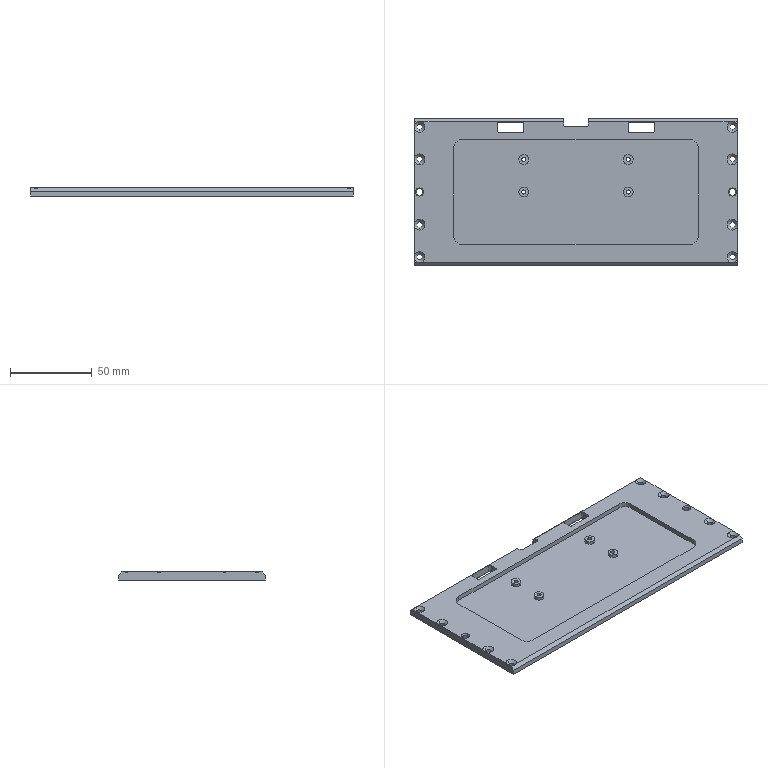Part | 1 solid | 322 faces | box 198 x 90 x 5 mm | volume 57298 mm3 | plane 164 | spline 80 | cylinder 50 | cone 28 | commonest cylinder face diameters 3.4 x16 2 x10 2.5 x8 6 x8 4 x4 12 x4